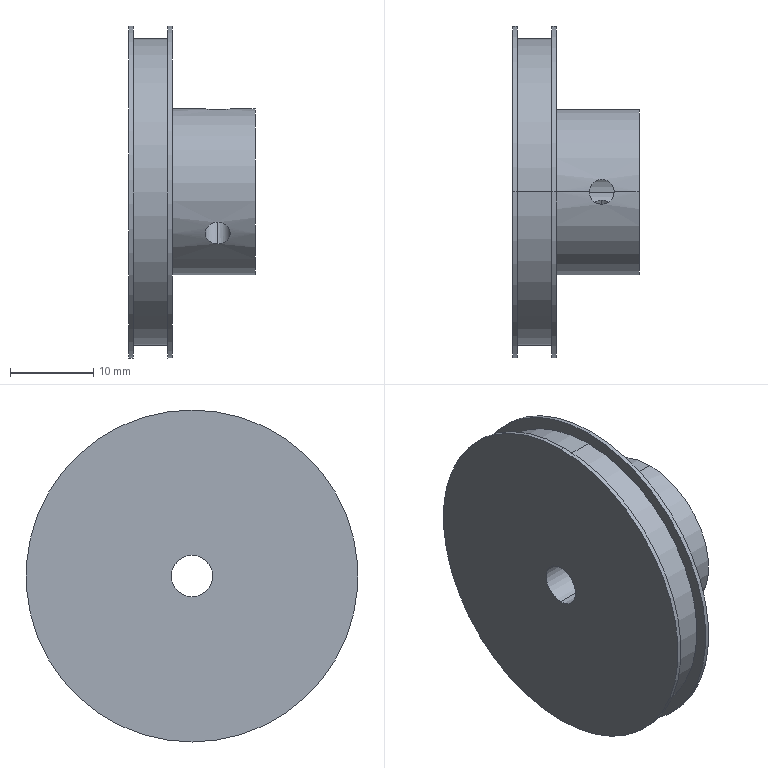Part | STEP file | Belt drive pulley | 1 solid | 19 faces | box 15.2 x 40 x 40 mm | volume 8508 mm3 | cylinder 14 | plane 5 | commonest cylinder face diameters 3 x4 40 x4 5 x2 20 x2 37 x2